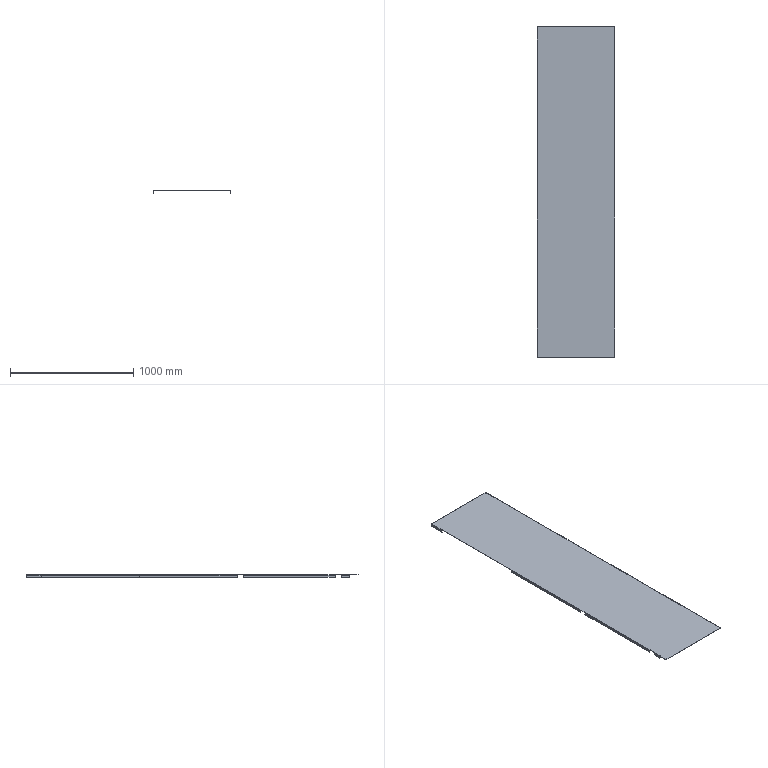Part | SolidWorks | features Cut 2, EdgeFlange 1, FlatPattern 1, SMBaseFlange 1, SheetMetal 1 | 1 solid | 78 faces | box 630 x 2698 x 20 mm | volume 2655544 mm3 | plane 62 | cylinder 16 | commonest cylinder face diameters 3 x8 6 x8